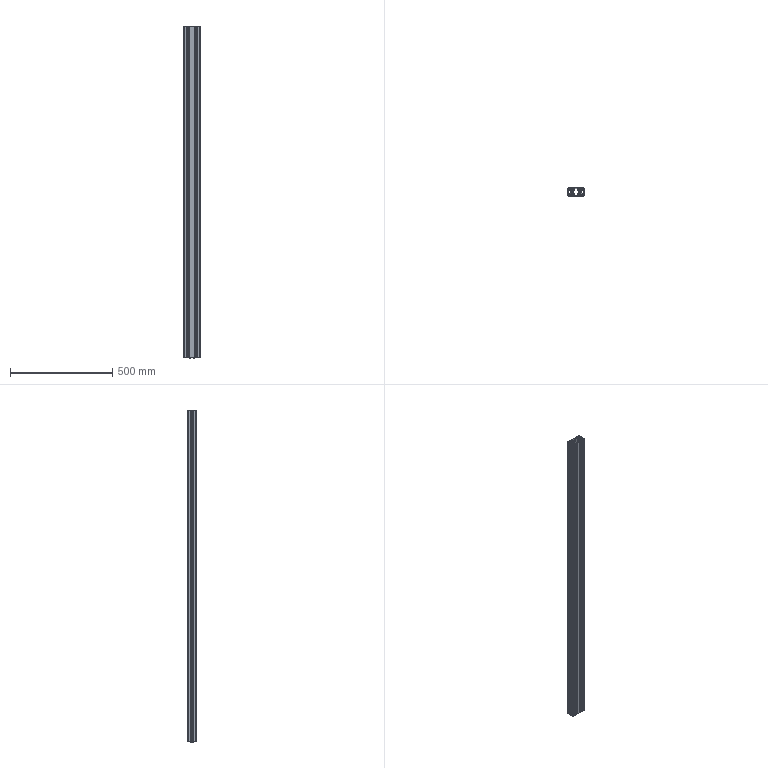Part | STEP file | HJLE-8-4080-S-OO_LE0724152727 | 1 solid | 286 faces | box 80 x 40 x 1620 mm | volume 1302826 mm3 | cylinder 144 | plane 142 | commonest cylinder face diameters 0.6 x48 2 x36 4 x28 0.4 x12 5 x4 6 x4